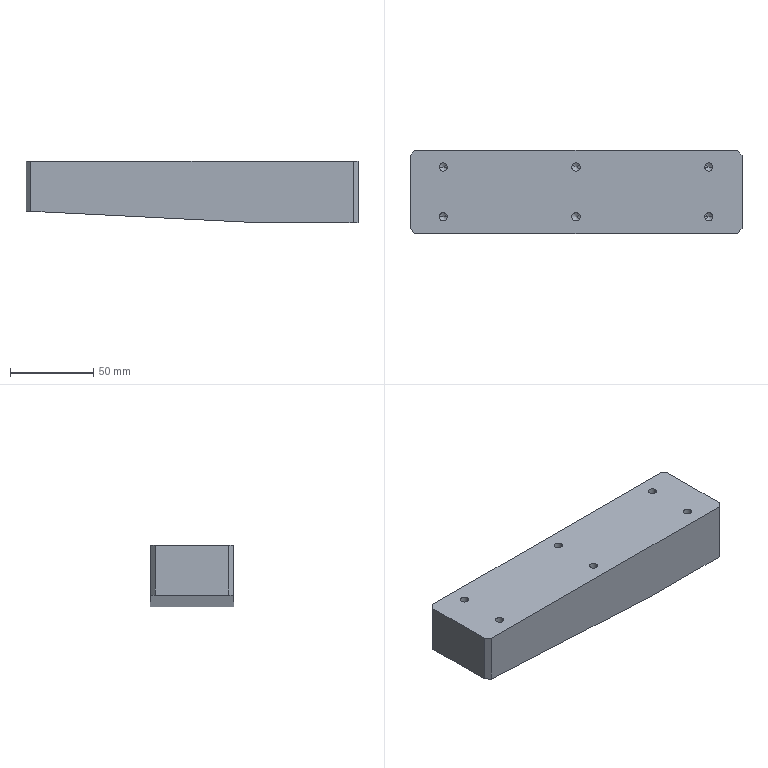Part | SolidWorks | features BaseBody 1 | 1 solid | 35 faces | box 200 x 50 x 37 mm | volume 343070 mm3 | cylinder 12 | cone 12 | plane 11 | commonest cylinder face diameters 5 x12
STEP:
#1=CARTESIAN_POINT('',(-82.5,15.,3.5));
#2=VERTEX_POINT('',#1);
#3=CARTESIAN_POINT('',(-77.5,15.,3.5));
#4=VERTEX_POINT('',#3);
#5=CARTESIAN_POINT('',(-80.,15.,3.5));
#6=DIRECTION('',(0.,0.,1.));
#7=DIRECTION('',(1.,0.,0.));
#8=AXIS2_PLACEMENT_3D('',#5,#6,#7);
#9=CIRCLE('',#8,2.5);
#10=EDGE_CURVE('',#2,#4,#9,.T.);
#11=ORIENTED_EDGE('',*,*,#10,.F.);
#12=CARTESIAN_POINT('',(-82.5,15.,18.5));
#13=VERTEX_POINT('',#12);
#14=CARTESIAN_POINT('',(-82.5,15.,18.5));
#15=DIRECTION('',(0.,0.,1.));
#16=VECTOR('',#15,1000.);
#17=LINE('',#14,#16);
#18=EDGE_CURVE('',#2,#13,#17,.T.);
#19=ORIENTED_EDGE('',*,*,#18,.T.);
#20=CARTESIAN_POINT('',(-77.5,15.,18.5));
#21=VERTEX_POINT('',#20);
#22=CARTESIAN_POINT('',(-80.,15.,18.5));
#23=DIRECTION('',(0.,0.,1.));
#24=DIRECTION('',(1.,0.,0.));
#25=AXIS2_PLACEMENT_3D('',#22,#23,#24);
#26=CIRCLE('',#25,2.5);
#27=EDGE_CURVE('',#13,#21,#26,.T.);
#28=ORIENTED_EDGE('',*,*,#27,.T.);
#29=CARTESIAN_POINT('',(-77.5,15.,18.5));
#30=DIRECTION('',(0.,0.,1.));
#31=VECTOR('',#30,1000.);
#32=LINE('',#29,#31);
#33=EDGE_CURVE('',#4,#21,#32,.T.);
#34=ORIENTED_EDGE('',*,*,#33,.F.);
#35=EDGE_LOOP('',(#11,#19,#28,#34));
#36=FACE_OUTER_BOUND('',#35,.T.);
#37=CARTESIAN_POINT('',(-80.,15.,18.5));
#38=DIRECTION('',(0.,0.,1.));
#39=DIRECTION('',(1.,0.,0.));
#40=AXIS2_PLACEMENT_3D('',#37,#38,#39);
#41=CYLINDRICAL_SURFACE('',#40,2.5);
#42=ADVANCED_FACE('',(#36),#41,.F.);
#43=CARTESIAN_POINT('',(-80.,15.,1.998));
#44=VERTEX_POINT('',#43);
#45=CARTESIAN_POINT('',(-77.5,15.,3.5));
#46=DIRECTION('',(0.8572,0.,0.515));
#47=VECTOR('',#46,1000.);
#48=LINE('',#45,#47);
#49=EDGE_CURVE('',#44,#4,#48,.T.);
#50=ORIENTED_EDGE('',*,*,#49,.F.);
#51=CARTESIAN_POINT('',(-82.5,15.,3.5));
#52=DIRECTION('',(-0.8572,0.,0.515));
#53=VECTOR('',#52,1000.);
#54=LINE('',#51,#53);
#55=EDGE_CURVE('',#44,#2,#54,.T.);
#56=ORIENTED_EDGE('',*,*,#55,.T.);
#57=ORIENTED_EDGE('',*,*,#10,.T.);
#58=EDGE_LOOP('',(#50,#56,#57));
#59=FACE_OUTER_BOUND('',#58,.T.);
#60=CARTESIAN_POINT('',(-80.,15.,3.5));
#61=DIRECTION('',(0.,0.,1.));
#62=DIRECTION('',(1.,0.,0.));
#63=AXIS2_PLACEMENT_3D('',#60,#61,#62);
#64=CONICAL_SURFACE('',#63,2.5,1.03);
#65=ADVANCED_FACE('',(#59),#64,.F.);
#66=CARTESIAN_POINT('',(-82.5,-15.,3.5));
#67=VERTEX_POINT('',#66);
#68=CARTESIAN_POINT('',(-77.5,-15.,3.5));
#69=VERTEX_POINT('',#68);
#70=CARTESIAN_POINT('',(-80.,-15.,3.5));
#71=DIRECTION('',(0.,0.,1.));
#72=DIRECTION('',(1.,0.,0.));
#73=AXIS2_PLACEMENT_3D('',#70,#71,#72);
#74=CIRCLE('',#73,2.5);
#75=EDGE_CURVE('',#67,#69,#74,.T.);
#76=ORIENTED_EDGE('',*,*,#75,.F.);
#77=CARTESIAN_POINT('',(-82.5,-15.,18.5));
#78=VERTEX_POINT('',#77);
#79=CARTESIAN_POINT('',(-82.5,-15.,18.5));
#80=DIRECTION('',(0.,0.,1.));
#81=VECTOR('',#80,1000.);
#82=LINE('',#79,#81);
#83=EDGE_CURVE('',#67,#78,#82,.T.);
#84=ORIENTED_EDGE('',*,*,#83,.T.);
#85=CARTESIAN_POINT('',(-77.5,-15.,18.5));
#86=VERTEX_POINT('',#85);
#87=CARTESIAN_POINT('',(-80.,-15.,18.5));
#88=DIRECTION('',(0.,0.,1.));
#89=DIRECTION('',(1.,0.,0.));
#90=AXIS2_PLACEMENT_3D('',#87,#88,#89);
#91=CIRCLE('',#90,2.5);
#92=EDGE_CURVE('',#78,#86,#91,.T.);
#93=ORIENTED_EDGE('',*,*,#92,.T.);
#94=CARTESIAN_POINT('',(-77.5,-15.,18.5));
#95=DIRECTION('',(0.,0.,1.));
#96=VECTOR('',#95,1000.);
#97=LINE('',#94,#96);
#98=EDGE_CURVE('',#69,#86,#97,.T.);
#99=ORIENTED_EDGE('',*,*,#98,.F.);
#100=EDGE_LOOP('',(#76,#84,#93,#99));
#101=FACE_OUTER_BOUND('',#100,.T.);
#102=CARTESIAN_POINT('',(-80.,-15.,18.5));
#103=DIRECTION('',(0.,0.,1.));
#104=DIRECTION('',(1.,0.,0.));
#105=AXIS2_PLACEMENT_3D('',#102,#103,#104);
#106=CYLINDRICAL_SURFACE('',#105,2.5);
#107=ADVANCED_FACE('',(#101),#106,.F.);
#108=CARTESIAN_POINT('',(-80.,-15.,1.998));
#109=VERTEX_POINT('',#108);
#110=CARTESIAN_POINT('',(-77.5,-15.,3.5));
#111=DIRECTION('',(0.8572,0.,0.515));
#112=VECTOR('',#111,1000.);
#113=LINE('',#110,#112);
#114=EDGE_CURVE('',#109,#69,#113,.T.);
#115=ORIENTED_EDGE('',*,*,#114,.F.);
#116=CARTESIAN_POINT('',(-82.5,-15.,3.5));
#117=DIRECTION('',(-0.8572,0.,0.515));
#118=VECTOR('',#117,1000.);
#119=LINE('',#116,#118);
#120=EDGE_CURVE('',#109,#67,#119,.T.);
#121=ORIENTED_EDGE('',*,*,#120,.T.);
#122=ORIENTED_EDGE('',*,*,#75,.T.);
#123=EDGE_LOOP('',(#115,#121,#122));
#124=FACE_OUTER_BOUND('',#123,.T.);
#125=CARTESIAN_POINT('',(-80.,-15.,3.5));
#126=DIRECTION('',(0.,0.,1.));
#127=DIRECTION('',(1.,0.,0.));
#128=AXIS2_PLACEMENT_3D('',#125,#126,#127);
#129=CONICAL_SURFACE('',#128,2.5,1.03);
#130=ADVANCED_FACE('',(#124),#129,.F.);
#131=CARTESIAN_POINT('',(-2.5,15.,3.5));
#132=VERTEX_POINT('',#131);
#133=CARTESIAN_POINT('',(2.5,15.,3.5));
#134=VERTEX_POINT('',#133);
#135=CARTESIAN_POINT('',(0.,15.,3.5));
#136=DIRECTION('',(0.,0.,1.));
#137=DIRECTION('',(1.,0.,0.));
#138=AXIS2_PLACEMENT_3D('',#135,#136,#137);
#139=CIRCLE('',#138,2.5);
#140=EDGE_CURVE('',#132,#134,#139,.T.);
#141=ORIENTED_EDGE('',*,*,#140,.F.);
#142=CARTESIAN_POINT('',(-2.5,15.,18.5));
#143=VERTEX_POINT('',#142);
#144=CARTESIAN_POINT('',(-2.5,15.,18.5));
#145=DIRECTION('',(0.,0.,1.));
#146=VECTOR('',#145,1000.);
#147=LINE('',#144,#146);
#148=EDGE_CURVE('',#132,#143,#147,.T.);
#149=ORIENTED_EDGE('',*,*,#148,.T.);
#150=CARTESIAN_POINT('',(2.5,15.,18.5));
#151=VERTEX_POINT('',#150);
#152=CARTESIAN_POINT('',(0.,15.,18.5));
#153=DIRECTION('',(0.,0.,1.));
#154=DIRECTION('',(1.,0.,0.));
#155=AXIS2_PLACEMENT_3D('',#152,#153,#154);
#156=CIRCLE('',#155,2.5);
#157=EDGE_CURVE('',#143,#151,#156,.T.);
#158=ORIENTED_EDGE('',*,*,#157,.T.);
#159=CARTESIAN_POINT('',(2.5,15.,18.5));
#160=DIRECTION('',(0.,0.,1.));
#161=VECTOR('',#160,1000.);
#162=LINE('',#159,#161);
#163=EDGE_CURVE('',#134,#151,#162,.T.);
#164=ORIENTED_EDGE('',*,*,#163,.F.);
#165=EDGE_LOOP('',(#141,#149,#158,#164));
#166=FACE_OUTER_BOUND('',#165,.T.);
#167=CARTESIAN_POINT('',(0.,15.,18.5));
#168=DIRECTION('',(0.,0.,1.));
#169=DIRECTION('',(1.,0.,0.));
#170=AXIS2_PLACEMENT_3D('',#167,#168,#169);
#171=CYLINDRICAL_SURFACE('',#170,2.5);
#172=ADVANCED_FACE('',(#166),#171,.F.);
#173=CARTESIAN_POINT('',(0.,15.,1.998));
#174=VERTEX_POINT('',#173);
#175=CARTESIAN_POINT('',(2.5,15.,3.5));
#176=DIRECTION('',(0.8572,0.,0.515));
#177=VECTOR('',#176,1000.);
#178=LINE('',#175,#177);
#179=EDGE_CURVE('',#174,#134,#178,.T.);
#180=ORIENTED_EDGE('',*,*,#179,.F.);
#181=CARTESIAN_POINT('',(-2.5,15.,3.5));
#182=DIRECTION('',(-0.8572,0.,0.515));
#183=VECTOR('',#182,1000.);
#184=LINE('',#181,#183);
#185=EDGE_CURVE('',#174,#132,#184,.T.);
#186=ORIENTED_EDGE('',*,*,#185,.T.);
#187=ORIENTED_EDGE('',*,*,#140,.T.);
#188=EDGE_LOOP('',(#180,#186,#187));
#189=FACE_OUTER_BOUND('',#188,.T.);
#190=CARTESIAN_POINT('',(0.,15.,3.5));
#191=DIRECTION('',(0.,0.,1.));
#192=DIRECTION('',(1.,0.,0.));
#193=AXIS2_PLACEMENT_3D('',#190,#191,#192);
#194=CONICAL_SURFACE('',#193,2.5,1.03);
#195=ADVANCED_FACE('',(#189),#194,.F.);
#196=CARTESIAN_POINT('',(-2.5,-15.,3.5));
#197=VERTEX_POINT('',#196);
#198=CARTESIAN_POINT('',(2.5,-15.,3.5));
#199=VERTEX_POINT('',#198);
#200=CARTESIAN_POINT('',(0.,-15.,3.5));
#201=DIRECTION('',(0.,0.,1.));
#202=DIRECTION('',(1.,0.,0.));
#203=AXIS2_PLACEMENT_3D('',#200,#201,#202);
#204=CIRCLE('',#203,2.5);
#205=EDGE_CURVE('',#197,#199,#204,.T.);
#206=ORIENTED_EDGE('',*,*,#205,.F.);
#207=CARTESIAN_POINT('',(-2.5,-15.,18.5));
#208=VERTEX_POINT('',#207);
#209=CARTESIAN_POINT('',(-2.5,-15.,18.5));
#210=DIRECTION('',(0.,0.,1.));
#211=VECTOR('',#210,1000.);
#212=LINE('',#209,#211);
#213=EDGE_CURVE('',#197,#208,#212,.T.);
#214=ORIENTED_EDGE('',*,*,#213,.T.);
#215=CARTESIAN_POINT('',(2.5,-15.,18.5));
#216=VERTEX_POINT('',#215);
#217=CARTESIAN_POINT('',(0.,-15.,18.5));
#218=DIRECTION('',(0.,0.,1.));
#219=DIRECTION('',(1.,0.,0.));
#220=AXIS2_PLACEMENT_3D('',#217,#218,#219);
#221=CIRCLE('',#220,2.5);
#222=EDGE_CURVE('',#208,#216,#221,.T.);
#223=ORIENTED_EDGE('',*,*,#222,.T.);
#224=CARTESIAN_POINT('',(2.5,-15.,18.5));
#225=DIRECTION('',(0.,0.,1.));
#226=VECTOR('',#225,1000.);
#227=LINE('',#224,#226);
#228=EDGE_CURVE('',#199,#216,#227,.T.);
#229=ORIENTED_EDGE('',*,*,#228,.F.);
#230=EDGE_LOOP('',(#206,#214,#223,#229));
#231=FACE_OUTER_BOUND('',#230,.T.);
#232=CARTESIAN_POINT('',(0.,-15.,18.5));
#233=DIRECTION('',(0.,0.,1.));
#234=DIRECTION('',(1.,0.,0.));
#235=AXIS2_PLACEMENT_3D('',#232,#233,#234);
#236=CYLINDRICAL_SURFACE('',#235,2.5);
#237=ADVANCED_FACE('',(#231),#236,.F.);
#238=CARTESIAN_POINT('',(0.,-15.,1.998));
#239=VERTEX_POINT('',#238);
#240=CARTESIAN_POINT('',(2.5,-15.,3.5));
#241=DIRECTION('',(0.8572,0.,0.515));
#242=VECTOR('',#241,1000.);
#243=LINE('',#240,#242);
#244=EDGE_CURVE('',#239,#199,#243,.T.);
#245=ORIENTED_EDGE('',*,*,#244,.F.);
#246=CARTESIAN_POINT('',(-2.5,-15.,3.5));
#247=DIRECTION('',(-0.8572,0.,0.515));
#248=VECTOR('',#247,1000.);
#249=LINE('',#246,#248);
#250=EDGE_CURVE('',#239,#197,#249,.T.);
#251=ORIENTED_EDGE('',*,*,#250,.T.);
#252=ORIENTED_EDGE('',*,*,#205,.T.);
#253=EDGE_LOOP('',(#245,#251,#252));
#254=FACE_OUTER_BOUND('',#253,.T.);
#255=CARTESIAN_POINT('',(0.,-15.,3.5));
#256=DIRECTION('',(0.,0.,1.));
#257=DIRECTION('',(1.,0.,0.));
#258=AXIS2_PLACEMENT_3D('',#255,#256,#257);
#259=CONICAL_SURFACE('',#258,2.5,1.03);
#260=ADVANCED_FACE('',(#254),#259,.F.);
#261=CARTESIAN_POINT('',(77.5,15.,3.5));
#262=VERTEX_POINT('',#261);
#263=CARTESIAN_POINT('',(82.5,15.,3.5));
#264=VERTEX_POINT('',#263);
#265=CARTESIAN_POINT('',(80.,15.,3.5));
#266=DIRECTION('',(0.,0.,1.));
#267=DIRECTION('',(1.,0.,0.));
#268=AXIS2_PLACEMENT_3D('',#265,#266,#267);
#269=CIRCLE('',#268,2.5);
#270=EDGE_CURVE('',#262,#264,#269,.T.);
#271=ORIENTED_EDGE('',*,*,#270,.F.);
#272=CARTESIAN_POINT('',(77.5,15.,18.5));
#273=VERTEX_POINT('',#272);
#274=CARTESIAN_POINT('',(77.5,15.,18.5));
#275=DIRECTION('',(0.,0.,1.));
#276=VECTOR('',#275,1000.);
#277=LINE('',#274,#276);
#278=EDGE_CURVE('',#262,#273,#277,.T.);
#279=ORIENTED_EDGE('',*,*,#278,.T.);
#280=CARTESIAN_POINT('',(82.5,15.,18.5));
#281=VERTEX_POINT('',#280);
#282=CARTESIAN_POINT('',(80.,15.,18.5));
#283=DIRECTION('',(0.,0.,1.));
#284=DIRECTION('',(1.,0.,0.));
#285=AXIS2_PLACEMENT_3D('',#282,#283,#284);
#286=CIRCLE('',#285,2.5);
#287=EDGE_CURVE('',#273,#281,#286,.T.);
#288=ORIENTED_EDGE('',*,*,#287,.T.);
#289=CARTESIAN_POINT('',(82.5,15.,18.5));
#290=DIRECTION('',(0.,0.,1.));
#291=VECTOR('',#290,1000.);
#292=LINE('',#289,#291);
#293=EDGE_CURVE('',#264,#281,#292,.T.);
#294=ORIENTED_EDGE('',*,*,#293,.F.);
#295=EDGE_LOOP('',(#271,#279,#288,#294));
#296=FACE_OUTER_BOUND('',#295,.T.);
#297=CARTESIAN_POINT('',(80.,15.,18.5));
#298=DIRECTION('',(0.,0.,1.));
#299=DIRECTION('',(1.,0.,0.));
#300=AXIS2_PLACEMENT_3D('',#297,#298,#299);
#301=CYLINDRICAL_SURFACE('',#300,2.5);
#302=ADVANCED_FACE('',(#296),#301,.F.);
#303=CARTESIAN_POINT('',(80.,15.,1.998));
#304=VERTEX_POINT('',#303);
#305=CARTESIAN_POINT('',(82.5,15.,3.5));
#306=DIRECTION('',(0.8572,0.,0.515));
#307=VECTOR('',#306,1000.);
#308=LINE('',#305,#307);
#309=EDGE_CURVE('',#304,#264,#308,.T.);
#310=ORIENTED_EDGE('',*,*,#309,.F.);
#311=CARTESIAN_POINT('',(77.5,15.,3.5));
#312=DIRECTION('',(-0.8572,0.,0.515));
#313=VECTOR('',#312,1000.);
#314=LINE('',#311,#313);
#315=EDGE_CURVE('',#304,#262,#314,.T.);
#316=ORIENTED_EDGE('',*,*,#315,.T.);
#317=ORIENTED_EDGE('',*,*,#270,.T.);
#318=EDGE_LOOP('',(#310,#316,#317));
#319=FACE_OUTER_BOUND('',#318,.T.);
#320=CARTESIAN_POINT('',(80.,15.,3.5));
#321=DIRECTION('',(0.,0.,1.));
#322=DIRECTION('',(1.,0.,0.));
#323=AXIS2_PLACEMENT_3D('',#320,#321,#322);
#324=CONICAL_SURFACE('',#323,2.5,1.03);
#325=ADVANCED_FACE('',(#319),#324,.F.);
#326=CARTESIAN_POINT('',(77.5,-15.,3.5));
#327=VERTEX_POINT('',#326);
#328=CARTESIAN_POINT('',(82.5,-15.,3.5));
#329=VERTEX_POINT('',#328);
#330=CARTESIAN_POINT('',(80.,-15.,3.5));
#331=DIRECTION('',(0.,0.,1.));
#332=DIRECTION('',(1.,0.,0.));
#333=AXIS2_PLACEMENT_3D('',#330,#331,#332);
#334=CIRCLE('',#333,2.5);
#335=EDGE_CURVE('',#327,#329,#334,.T.);
#336=ORIENTED_EDGE('',*,*,#335,.F.);
#337=CARTESIAN_POINT('',(77.5,-15.,18.5));
#338=VERTEX_POINT('',#337);
#339=CARTESIAN_POINT('',(77.5,-15.,18.5));
#340=DIRECTION('',(0.,0.,1.));
#341=VECTOR('',#340,1000.);
#342=LINE('',#339,#341);
#343=EDGE_CURVE('',#327,#338,#342,.T.);
#344=ORIENTED_EDGE('',*,*,#343,.T.);
#345=CARTESIAN_POINT('',(82.5,-15.,18.5));
#346=VERTEX_POINT('',#345);
#347=CARTESIAN_POINT('',(80.,-15.,18.5));
#348=DIRECTION('',(0.,0.,1.));
#349=DIRECTION('',(1.,0.,0.));
#350=AXIS2_PLACEMENT_3D('',#347,#348,#349);
#351=CIRCLE('',#350,2.5);
#352=EDGE_CURVE('',#338,#346,#351,.T.);
#353=ORIENTED_EDGE('',*,*,#352,.T.);
#354=CARTESIAN_POINT('',(82.5,-15.,18.5));
#355=DIRECTION('',(0.,0.,1.));
#356=VECTOR('',#355,1000.);
#357=LINE('',#354,#356);
#358=EDGE_CURVE('',#329,#346,#357,.T.);
#359=ORIENTED_EDGE('',*,*,#358,.F.);
#360=EDGE_LOOP('',(#336,#344,#353,#359));
#361=FACE_OUTER_BOUND('',#360,.T.);
#362=CARTESIAN_POINT('',(80.,-15.,18.5));
#363=DIRECTION('',(0.,0.,1.));
#364=DIRECTION('',(1.,0.,0.));
#365=AXIS2_PLACEMENT_3D('',#362,#363,#364);
#366=CYLINDRICAL_SURFACE('',#365,2.5);
#367=ADVANCED_FACE('',(#361),#366,.F.);
#368=CARTESIAN_POINT('',(80.,-15.,1.998));
#369=VERTEX_POINT('',#368);
#370=CARTESIAN_POINT('',(82.5,-15.,3.5));
#371=DIRECTION('',(0.8572,0.,0.515));
#372=VECTOR('',#371,1000.);
#373=LINE('',#370,#372);
#374=EDGE_CURVE('',#369,#329,#373,.T.);
#375=ORIENTED_EDGE('',*,*,#374,.F.);
#376=CARTESIAN_POINT('',(77.5,-15.,3.5));
#377=DIRECTION('',(-0.8572,0.,0.515));
#378=VECTOR('',#377,1000.);
#379=LINE('',#376,#378);
#380=EDGE_CURVE('',#369,#327,#379,.T.);
#381=ORIENTED_EDGE('',*,*,#380,.T.);
#382=ORIENTED_EDGE('',*,*,#335,.T.);
#383=EDGE_LOOP('',(#375,#381,#382));
#384=FACE_OUTER_BOUND('',#383,.T.);
#385=CARTESIAN_POINT('',(80.,-15.,3.5));
#386=DIRECTION('',(0.,0.,1.));
#387=DIRECTION('',(1.,0.,0.));
#388=AXIS2_PLACEMENT_3D('',#385,#386,#387);
#389=CONICAL_SURFACE('',#388,2.5,1.03);
#390=ADVANCED_FACE('',(#384),#389,.F.);
#391=CARTESIAN_POINT('',(-100.,-22.,-11.5));
#392=VERTEX_POINT('',#391);
#393=CARTESIAN_POINT('',(-100.,22.,-11.5));
#394=VERTEX_POINT('',#393);
#395=CARTESIAN_POINT('',(-100.,-25.,-11.5));
#396=DIRECTION('',(0.,1.,0.));
#397=VECTOR('',#396,1000.);
#398=LINE('',#395,#397);
#399=EDGE_CURVE('',#392,#394,#398,.T.);
#400=ORIENTED_EDGE('',*,*,#399,.F.);
#401=CARTESIAN_POINT('',(-100.,-22.,18.5));
#402=VERTEX_POINT('',#401);
#403=CARTESIAN_POINT('',(-100.,-22.,18.5));
#404=DIRECTION('',(0.,0.,1.));
#405=VECTOR('',#404,1000.);
#406=LINE('',#403,#405);
#407=EDGE_CURVE('',#392,#402,#406,.T.);
#408=ORIENTED_EDGE('',*,*,#407,.T.);
#409=CARTESIAN_POINT('',(-100.,22.,18.5));
#410=VERTEX_POINT('',#409);
#411=CARTESIAN_POINT('',(-100.,25.,18.5));
#412=DIRECTION('',(0.,-1.,0.));
#413=VECTOR('',#412,1000.);
#414=LINE('',#411,#413);
#415=EDGE_CURVE('',#410,#402,#414,.T.);
#416=ORIENTED_EDGE('',*,*,#415,.F.);
#417=CARTESIAN_POINT('',(-100.,22.,18.5));
#418=DIRECTION('',(0.,0.,-1.));
#419=VECTOR('',#418,1000.);
#420=LINE('',#417,#419);
#421=EDGE_CURVE('',#410,#394,#420,.T.);
#422=ORIENTED_EDGE('',*,*,#421,.T.);
#423=EDGE_LOOP('',(#400,#408,#416,#422));
#424=FACE_OUTER_BOUND('',#423,.T.);
#425=CARTESIAN_POINT('',(-100.,25.,18.5));
#426=DIRECTION('',(1.,0.,0.));
#427=DIRECTION('',(0.,0.,-1.));
#428=AXIS2_PLACEMENT_3D('',#425,#426,#427);
#429=PLANE('',#428);
#430=ADVANCED_FACE('',(#424),#429,.F.);
#431=CARTESIAN_POINT('',(40.,-25.,-18.5));
#432=VERTEX_POINT('',#431);
#433=CARTESIAN_POINT('',(97.,-25.,-18.5));
#434=VERTEX_POINT('',#433);
#435=CARTESIAN_POINT('',(100.,-25.,-18.5));
#436=DIRECTION('',(1.,0.,0.));
#437=VECTOR('',#436,1000.);
#438=LINE('',#435,#437);
#439=EDGE_CURVE('',#432,#434,#438,.T.);
#440=ORIENTED_EDGE('',*,*,#439,.T.);
#441=CARTESIAN_POINT('',(97.,-25.,18.5));
#442=VERTEX_POINT('',#441);
#443=CARTESIAN_POINT('',(97.,-25.,18.5));
#444=DIRECTION('',(0.,0.,1.));
#445=VECTOR('',#444,1000.);
#446=LINE('',#443,#445);
#447=EDGE_CURVE('',#434,#442,#446,.T.);
#448=ORIENTED_EDGE('',*,*,#447,.T.);
#449=CARTESIAN_POINT('',(-97.,-25.,18.5));
#450=VERTEX_POINT('',#449);
#451=CARTESIAN_POINT('',(100.,-25.,18.5));
#452=DIRECTION('',(1.,0.,0.));
#453=VECTOR('',#452,1000.);
#454=LINE('',#451,#453);
#455=EDGE_CURVE('',#450,#442,#454,.T.);
#456=ORIENTED_EDGE('',*,*,#455,.F.);
#457=CARTESIAN_POINT('',(-97.,-25.,-11.65));
#458=VERTEX_POINT('',#457);
#459=CARTESIAN_POINT('',(-97.,-25.,18.5));
#460=DIRECTION('',(0.,0.,-1.));
#461=VECTOR('',#460,1000.);
#462=LINE('',#459,#461);
#463=EDGE_CURVE('',#450,#458,#462,.T.);
#464=ORIENTED_EDGE('',*,*,#463,.T.);
#465=CARTESIAN_POINT('',(-100.,-25.,-11.5));
#466=DIRECTION('',(0.9988,0.,-0.04994));
#467=VECTOR('',#466,1000.);
#468=LINE('',#465,#467);
#469=EDGE_CURVE('',#458,#432,#468,.T.);
#470=ORIENTED_EDGE('',*,*,#469,.T.);
#471=EDGE_LOOP('',(#440,#448,#456,#464,#470));
#472=FACE_OUTER_BOUND('',#471,.T.);
#473=CARTESIAN_POINT('',(100.,-25.,18.5));
#474=DIRECTION('',(0.,1.,0.));
#475=DIRECTION('',(-1.,0.,0.));
#476=AXIS2_PLACEMENT_3D('',#473,#474,#475);
#477=PLANE('',#476);
#478=ADVANCED_FACE('',(#472),#477,.F.);
#479=CARTESIAN_POINT('',(100.,-22.,18.5));
#480=VERTEX_POINT('',#479);
#481=CARTESIAN_POINT('',(100.,22.,18.5));
#482=VERTEX_POINT('',#481);
#483=CARTESIAN_POINT('',(100.,25.,18.5));
#484=DIRECTION('',(0.,1.,0.));
#485=VECTOR('',#484,1000.);
#486=LINE('',#483,#485);
#487=EDGE_CURVE('',#480,#482,#486,.T.);
#488=ORIENTED_EDGE('',*,*,#487,.F.);
#489=CARTESIAN_POINT('',(100.,-22.,-18.5));
#490=VERTEX_POINT('',#489);
#491=CARTESIAN_POINT('',(100.,-22.,18.5));
#492=DIRECTION('',(0.,0.,-1.));
#493=VECTOR('',#492,1000.);
#494=LINE('',#491,#493);
#495=EDGE_CURVE('',#480,#490,#494,.T.);
#496=ORIENTED_EDGE('',*,*,#495,.T.);
#497=CARTESIAN_POINT('',(100.,22.,-18.5));
#498=VERTEX_POINT('',#497);
#499=CARTESIAN_POINT('',(100.,25.,-18.5));
#500=DIRECTION('',(0.,1.,0.));
#501=VECTOR('',#500,1000.);
#502=LINE('',#499,#501);
#503=EDGE_CURVE('',#490,#498,#502,.T.);
#504=ORIENTED_EDGE('',*,*,#503,.T.);
#505=CARTESIAN_POINT('',(100.,22.,18.5));
#506=DIRECTION('',(0.,0.,1.));
#507=VECTOR('',#506,1000.);
#508=LINE('',#505,#507);
#509=EDGE_CURVE('',#498,#482,#508,.T.);
#510=ORIENTED_EDGE('',*,*,#509,.T.);
#511=EDGE_LOOP('',(#488,#496,#504,#510));
#512=FACE_OUTER_BOUND('',#511,.T.);
#513=CARTESIAN_POINT('',(100.,25.,18.5));
#514=DIRECTION('',(-1.,0.,0.));
#515=DIRECTION('',(0.,0.,1.));
#516=AXIS2_PLACEMENT_3D('',#513,#514,#515);
#517=PLANE('',#516);
#518=ADVANCED_FACE('',(#512),#517,.F.);
#519=CARTESIAN_POINT('',(97.,25.,18.5));
#520=VERTEX_POINT('',#519);
#521=CARTESIAN_POINT('',(-97.,25.,18.5));
#522=VERTEX_POINT('',#521);
#523=CARTESIAN_POINT('',(100.,25.,18.5));
#524=DIRECTION('',(-1.,0.,0.));
#525=VECTOR('',#524,1000.);
#526=LINE('',#523,#525);
#527=EDGE_CURVE('',#520,#522,#526,.T.);
#528=ORIENTED_EDGE('',*,*,#527,.F.);
#529=CARTESIAN_POINT('',(97.,25.,-18.5));
#530=VERTEX_POINT('',#529);
#531=CARTESIAN_POINT('',(97.,25.,18.5));
#532=DIRECTION('',(0.,0.,-1.));
#533=VECTOR('',#532,1000.);
#534=LINE('',#531,#533);
#535=EDGE_CURVE('',#520,#530,#534,.T.);
#536=ORIENTED_EDGE('',*,*,#535,.T.);
#537=CARTESIAN_POINT('',(40.,25.,-18.5));
#538=VERTEX_POINT('',#537);
#539=CARTESIAN_POINT('',(100.,25.,-18.5));
#540=DIRECTION('',(-1.,0.,0.));
#541=VECTOR('',#540,1000.);
#542=LINE('',#539,#541);
#543=EDGE_CURVE('',#530,#538,#542,.T.);
#544=ORIENTED_EDGE('',*,*,#543,.T.);
#545=CARTESIAN_POINT('',(-97.,25.,-11.65));
#546=VERTEX_POINT('',#545);
#547=CARTESIAN_POINT('',(-100.,25.,-11.5));
#548=DIRECTION('',(0.9988,0.,-0.04994));
#549=VECTOR('',#548,1000.);
#550=LINE('',#547,#549);
#551=EDGE_CURVE('',#546,#538,#550,.T.);
#552=ORIENTED_EDGE('',*,*,#551,.F.);
#553=CARTESIAN_POINT('',(-97.,25.,18.5));
#554=DIRECTION('',(0.,0.,1.));
#555=VECTOR('',#554,1000.);
#556=LINE('',#553,#555);
#557=EDGE_CURVE('',#546,#522,#556,.T.);
#558=ORIENTED_EDGE('',*,*,#557,.T.);
#559=EDGE_LOOP('',(#528,#536,#544,#552,#558));
#560=FACE_OUTER_BOUND('',#559,.T.);
#561=CARTESIAN_POINT('',(100.,25.,18.5));
#562=DIRECTION('',(0.,-1.,0.));
#563=DIRECTION('',(1.,0.,0.));
#564=AXIS2_PLACEMENT_3D('',#561,#562,#563);
#565=PLANE('',#564);
#566=ADVANCED_FACE('',(#560),#565,.F.);
#567=CARTESIAN_POINT('',(-80.,15.,18.5));
#568=DIRECTION('',(0.,0.,1.));
#569=DIRECTION('',(1.,0.,0.));
#570=AXIS2_PLACEMENT_3D('',#567,#568,#569);
#571=CIRCLE('',#570,2.5);
#572=EDGE_CURVE('',#21,#13,#571,.T.);
#573=ORIENTED_EDGE('',*,*,#572,.F.);
#574=ORIENTED_EDGE('',*,*,#27,.F.);
#575=EDGE_LOOP('',(#573,#574));
#576=FACE_BOUND('',#575,.T.);
#577=CARTESIAN_POINT('',(-80.,-15.,18.5));
#578=DIRECTION('',(0.,0.,1.));
#579=DIRECTION('',(1.,0.,0.));
#580=AXIS2_PLACEMENT_3D('',#577,#578,#579);
#581=CIRCLE('',#580,2.5);
#582=EDGE_CURVE('',#86,#78,#581,.T.);
#583=ORIENTED_EDGE('',*,*,#582,.F.);
#584=ORIENTED_EDGE('',*,*,#92,.F.);
#585=EDGE_LOOP('',(#583,#584));
#586=FACE_BOUND('',#585,.T.);
#587=CARTESIAN_POINT('',(0.,15.,18.5));
#588=DIRECTION('',(0.,0.,1.));
#589=DIRECTION('',(1.,0.,0.));
#590=AXIS2_PLACEMENT_3D('',#587,#588,#589);
#591=CIRCLE('',#590,2.5);
#592=EDGE_CURVE('',#151,#143,#591,.T.);
#593=ORIENTED_EDGE('',*,*,#592,.F.);
#594=ORIENTED_EDGE('',*,*,#157,.F.);
#595=EDGE_LOOP('',(#593,#594));
#596=FACE_BOUND('',#595,.T.);
#597=CARTESIAN_POINT('',(0.,-15.,18.5));
#598=DIRECTION('',(0.,0.,1.));
#599=DIRECTION('',(1.,0.,0.));
#600=AXIS2_PLACEMENT_3D('',#597,#598,#599);
#601=CIRCLE('',#600,2.5);
#602=EDGE_CURVE('',#216,#208,#601,.T.);
#603=ORIENTED_EDGE('',*,*,#602,.F.);
#604=ORIENTED_EDGE('',*,*,#222,.F.);
#605=EDGE_LOOP('',(#603,#604));
#606=FACE_BOUND('',#605,.T.);
#607=CARTESIAN_POINT('',(80.,15.,18.5));
#608=DIRECTION('',(0.,0.,1.));
#609=DIRECTION('',(1.,0.,0.));
#610=AXIS2_PLACEMENT_3D('',#607,#608,#609);
#611=CIRCLE('',#610,2.5);
#612=EDGE_CURVE('',#281,#273,#611,.T.);
#613=ORIENTED_EDGE('',*,*,#612,.F.);
#614=ORIENTED_EDGE('',*,*,#287,.F.);
#615=EDGE_LOOP('',(#613,#614));
#616=FACE_BOUND('',#615,.T.);
#617=CARTESIAN_POINT('',(80.,-15.,18.5));
#618=DIRECTION('',(0.,0.,1.));
#619=DIRECTION('',(1.,0.,0.));
#620=AXIS2_PLACEMENT_3D('',#617,#618,#619);
#621=CIRCLE('',#620,2.5);
#622=EDGE_CURVE('',#346,#338,#621,.T.);
#623=ORIENTED_EDGE('',*,*,#622,.F.);
#624=ORIENTED_EDGE('',*,*,#352,.F.);
#625=EDGE_LOOP('',(#623,#624));
#626=FACE_BOUND('',#625,.T.);
#627=ORIENTED_EDGE('',*,*,#455,.T.);
#628=CARTESIAN_POINT('',(100.,-22.,18.5));
#629=DIRECTION('',(0.7071,0.7071,0.));
#630=VECTOR('',#629,1000.);
#631=LINE('',#628,#630);
#632=EDGE_CURVE('',#442,#480,#631,.T.);
#633=ORIENTED_EDGE('',*,*,#632,.T.);
#634=ORIENTED_EDGE('',*,*,#487,.T.);
#635=CARTESIAN_POINT('',(97.,25.,18.5));
#636=DIRECTION('',(-0.7071,0.7071,0.));
#637=VECTOR('',#636,1000.);
#638=LINE('',#635,#637);
#639=EDGE_CURVE('',#482,#520,#638,.T.);
#640=ORIENTED_EDGE('',*,*,#639,.T.);
#641=ORIENTED_EDGE('',*,*,#527,.T.);
#642=CARTESIAN_POINT('',(-100.,22.,18.5));
#643=DIRECTION('',(-0.7071,-0.7071,0.));
#644=VECTOR('',#643,1000.);
#645=LINE('',#642,#644);
#646=EDGE_CURVE('',#522,#410,#645,.T.);
#647=ORIENTED_EDGE('',*,*,#646,.T.);
#648=ORIENTED_EDGE('',*,*,#415,.T.);
#649=CARTESIAN_POINT('',(-97.,-25.,18.5));
#650=DIRECTION('',(0.7071,-0.7071,0.));
#651=VECTOR('',#650,1000.);
#652=LINE('',#649,#651);
#653=EDGE_CURVE('',#402,#450,#652,.T.);
#654=ORIENTED_EDGE('',*,*,#653,.T.);
#655=EDGE_LOOP('',(#627,#633,#634,#640,#641,#647,#648,#654));
#656=FACE_OUTER_BOUND('',#655,.T.);
#657=CARTESIAN_POINT('',(-100.,-25.,18.5));
#658=DIRECTION('',(0.,0.,-1.));
#659=DIRECTION('',(-1.,0.,0.));
#660=AXIS2_PLACEMENT_3D('',#657,#658,#659);
#661=PLANE('',#660);
#662=ADVANCED_FACE('',(#576,#586,#596,#606,#616,#626,#656),#661,.F.);
#663=ORIENTED_EDGE('',*,*,#503,.F.);
#664=CARTESIAN_POINT('',(-1.5,-123.5,-18.5));
#665=DIRECTION('',(-0.7071,-0.7071,0.));
#666=VECTOR('',#665,1000.);
#667=LINE('',#664,#666);
#668=EDGE_CURVE('',#490,#434,#667,.T.);
#669=ORIENTED_EDGE('',*,*,#668,.T.);
#670=ORIENTED_EDGE('',*,*,#439,.F.);
#671=CARTESIAN_POINT('',(40.,-25.,-18.5));
#672=DIRECTION('',(0.,1.,0.));
#673=VECTOR('',#672,1000.);
#674=LINE('',#671,#673);
#675=EDGE_CURVE('',#432,#538,#674,.T.);
#676=ORIENTED_EDGE('',*,*,#675,.T.);
#677=ORIENTED_EDGE('',*,*,#543,.F.);
#678=CARTESIAN_POINT('',(23.5,98.5,-18.5));
#679=DIRECTION('',(0.7071,-0.7071,0.));
#680=VECTOR('',#679,1000.);
#681=LINE('',#678,#680);
#682=EDGE_CURVE('',#530,#498,#681,.T.);
#683=ORIENTED_EDGE('',*,*,#682,.T.);
#684=EDGE_LOOP('',(#663,#669,#670,#676,#677,#683));
#685=FACE_OUTER_BOUND('',#684,.T.);
#686=CARTESIAN_POINT('',(-100.,-25.,-18.5));
#687=DIRECTION('',(0.,0.,-1.));
#688=DIRECTION('',(-1.,0.,0.));
#689=AXIS2_PLACEMENT_3D('',#686,#687,#688);
#690=PLANE('',#689);
#691=ADVANCED_FACE('',(#685),#690,.T.);
#692=ORIENTED_EDGE('',*,*,#469,.F.);
#693=CARTESIAN_POINT('',(-97.753,-24.247,-11.612));
#694=DIRECTION('',(-0.7067,0.7067,0.03533));
#695=VECTOR('',#694,1000.);
#696=LINE('',#693,#695);
#697=EDGE_CURVE('',#458,#392,#696,.T.);
#698=ORIENTED_EDGE('',*,*,#697,.T.);
#699=ORIENTED_EDGE('',*,*,#399,.T.);
#700=CARTESIAN_POINT('',(-100.749,21.251,-11.463));
#701=DIRECTION('',(0.7067,0.7067,-0.03533));
#702=VECTOR('',#701,1000.);
#703=LINE('',#700,#702);
#704=EDGE_CURVE('',#394,#546,#703,.T.);
#705=ORIENTED_EDGE('',*,*,#704,.T.);
#706=ORIENTED_EDGE('',*,*,#551,.T.);
#707=ORIENTED_EDGE('',*,*,#675,.F.);
#708=EDGE_LOOP('',(#692,#698,#699,#705,#706,#707));
#709=FACE_OUTER_BOUND('',#708,.T.);
#710=CARTESIAN_POINT('',(-100.,-25.,-11.5));
#711=DIRECTION('',(0.04994,0.,0.9988));
#712=DIRECTION('',(0.9988,0.,-0.04994));
#713=AXIS2_PLACEMENT_3D('',#710,#711,#712);
#714=PLANE('',#713);
#715=ADVANCED_FACE('',(#709),#714,.F.);
#716=ORIENTED_EDGE('',*,*,#632,.F.);
#717=ORIENTED_EDGE('',*,*,#447,.F.);
#718=ORIENTED_EDGE('',*,*,#668,.F.);
#719=ORIENTED_EDGE('',*,*,#495,.F.);
#720=EDGE_LOOP('',(#716,#717,#718,#719));
#721=FACE_OUTER_BOUND('',#720,.T.);
#722=CARTESIAN_POINT('',(100.,-22.,18.5));
#723=DIRECTION('',(-0.7071,0.7071,0.));
#724=DIRECTION('',(-0.7071,-0.7071,0.));
#725=AXIS2_PLACEMENT_3D('',#722,#723,#724);
#726=PLANE('',#725);
#727=ADVANCED_FACE('',(#721),#726,.F.);
#728=ORIENTED_EDGE('',*,*,#639,.F.);
#729=ORIENTED_EDGE('',*,*,#509,.F.);
#730=ORIENTED_EDGE('',*,*,#682,.F.);
#731=ORIENTED_EDGE('',*,*,#535,.F.);
#732=EDGE_LOOP('',(#728,#729,#730,#731));
#733=FACE_OUTER_BOUND('',#732,.T.);
#734=CARTESIAN_POINT('',(97.,25.,18.5));
#735=DIRECTION('',(-0.7071,-0.7071,0.));
#736=DIRECTION('',(0.7071,-0.7071,0.));
#737=AXIS2_PLACEMENT_3D('',#734,#735,#736);
#738=PLANE('',#737);
#739=ADVANCED_FACE('',(#733),#738,.F.);
#740=ORIENTED_EDGE('',*,*,#653,.F.);
#741=ORIENTED_EDGE('',*,*,#407,.F.);
#742=ORIENTED_EDGE('',*,*,#697,.F.);
#743=ORIENTED_EDGE('',*,*,#463,.F.);
#744=EDGE_LOOP('',(#740,#741,#742,#743));
#745=FACE_OUTER_BOUND('',#744,.T.);
#746=CARTESIAN_POINT('',(-97.,-25.,18.5));
#747=DIRECTION('',(0.7071,0.7071,0.));
#748=DIRECTION('',(-0.7071,0.7071,0.));
#749=AXIS2_PLACEMENT_3D('',#746,#747,#748);
#750=PLANE('',#749);
#751=ADVANCED_FACE('',(#745),#750,.F.);
#752=ORIENTED_EDGE('',*,*,#646,.F.);
#753=ORIENTED_EDGE('',*,*,#557,.F.);
#754=ORIENTED_EDGE('',*,*,#704,.F.);
#755=ORIENTED_EDGE('',*,*,#421,.F.);
#756=EDGE_LOOP('',(#752,#753,#754,#755));
#757=FACE_OUTER_BOUND('',#756,.T.);
#758=CARTESIAN_POINT('',(-100.,22.,18.5));
#759=DIRECTION('',(0.7071,-0.7071,0.));
#760=DIRECTION('',(0.7071,0.7071,0.));
#761=AXIS2_PLACEMENT_3D('',#758,#759,#760);
#762=PLANE('',#761);
#763=ADVANCED_FACE('',(#757),#762,.F.);
#764=ORIENTED_EDGE('',*,*,#380,.F.);
#765=ORIENTED_EDGE('',*,*,#374,.T.);
#766=CARTESIAN_POINT('',(80.,-15.,3.5));
#767=DIRECTION('',(0.,0.,1.));
#768=DIRECTION('',(1.,0.,0.));
#769=AXIS2_PLACEMENT_3D('',#766,#767,#768);
#770=CIRCLE('',#769,2.5);
#771=EDGE_CURVE('',#329,#327,#770,.T.);
#772=ORIENTED_EDGE('',*,*,#771,.T.);
#773=EDGE_LOOP('',(#764,#765,#772));
#774=FACE_OUTER_BOUND('',#773,.T.);
#775=CARTESIAN_POINT('',(80.,-15.,3.5));
#776=DIRECTION('',(0.,0.,1.));
#777=DIRECTION('',(1.,0.,0.));
#778=AXIS2_PLACEMENT_3D('',#775,#776,#777);
#779=CONICAL_SURFACE('',#778,2.5,1.03);
#780=ADVANCED_FACE('',(#774),#779,.F.);
#781=ORIENTED_EDGE('',*,*,#343,.F.);
#782=ORIENTED_EDGE('',*,*,#771,.F.);
#783=ORIENTED_EDGE('',*,*,#358,.T.);
#784=ORIENTED_EDGE('',*,*,#622,.T.);
#785=EDGE_LOOP('',(#781,#782,#783,#784));
#786=FACE_OUTER_BOUND('',#785,.T.);
#787=CARTESIAN_POINT('',(80.,-15.,18.5));
#788=DIRECTION('',(0.,0.,1.));
#789=DIRECTION('',(1.,0.,0.));
#790=AXIS2_PLACEMENT_3D('',#787,#788,#789);
#791=CYLINDRICAL_SURFACE('',#790,2.5);
#792=ADVANCED_FACE('',(#786),#791,.F.);
#793=ORIENTED_EDGE('',*,*,#315,.F.);
#794=ORIENTED_EDGE('',*,*,#309,.T.);
#795=CARTESIAN_POINT('',(80.,15.,3.5));
#796=DIRECTION('',(0.,0.,1.));
#797=DIRECTION('',(1.,0.,0.));
#798=AXIS2_PLACEMENT_3D('',#795,#796,#797);
#799=CIRCLE('',#798,2.5);
#800=EDGE_CURVE('',#264,#262,#799,.T.);
#801=ORIENTED_EDGE('',*,*,#800,.T.);
#802=EDGE_LOOP('',(#793,#794,#801));
#803=FACE_OUTER_BOUND('',#802,.T.);
#804=CARTESIAN_POINT('',(80.,15.,3.5));
#805=DIRECTION('',(0.,0.,1.));
#806=DIRECTION('',(1.,0.,0.));
#807=AXIS2_PLACEMENT_3D('',#804,#805,#806);
#808=CONICAL_SURFACE('',#807,2.5,1.03);
#809=ADVANCED_FACE('',(#803),#808,.F.);
#810=ORIENTED_EDGE('',*,*,#278,.F.);
#811=ORIENTED_EDGE('',*,*,#800,.F.);
#812=ORIENTED_EDGE('',*,*,#293,.T.);
#813=ORIENTED_EDGE('',*,*,#612,.T.);
#814=EDGE_LOOP('',(#810,#811,#812,#813));
#815=FACE_OUTER_BOUND('',#814,.T.);
#816=CARTESIAN_POINT('',(80.,15.,18.5));
#817=DIRECTION('',(0.,0.,1.));
#818=DIRECTION('',(1.,0.,0.));
#819=AXIS2_PLACEMENT_3D('',#816,#817,#818);
#820=CYLINDRICAL_SURFACE('',#819,2.5);
#821=ADVANCED_FACE('',(#815),#820,.F.);
#822=ORIENTED_EDGE('',*,*,#250,.F.);
#823=ORIENTED_EDGE('',*,*,#244,.T.);
#824=CARTESIAN_POINT('',(0.,-15.,3.5));
#825=DIRECTION('',(0.,0.,1.));
#826=DIRECTION('',(1.,0.,0.));
#827=AXIS2_PLACEMENT_3D('',#824,#825,#826);
#828=CIRCLE('',#827,2.5);
#829=EDGE_CURVE('',#199,#197,#828,.T.);
#830=ORIENTED_EDGE('',*,*,#829,.T.);
#831=EDGE_LOOP('',(#822,#823,#830));
#832=FACE_OUTER_BOUND('',#831,.T.);
#833=CARTESIAN_POINT('',(0.,-15.,3.5));
#834=DIRECTION('',(0.,0.,1.));
#835=DIRECTION('',(1.,0.,0.));
#836=AXIS2_PLACEMENT_3D('',#833,#834,#835);
#837=CONICAL_SURFACE('',#836,2.5,1.03);
#838=ADVANCED_FACE('',(#832),#837,.F.);
#839=ORIENTED_EDGE('',*,*,#213,.F.);
#840=ORIENTED_EDGE('',*,*,#829,.F.);
#841=ORIENTED_EDGE('',*,*,#228,.T.);
#842=ORIENTED_EDGE('',*,*,#602,.T.);
#843=EDGE_LOOP('',(#839,#840,#841,#842));
#844=FACE_OUTER_BOUND('',#843,.T.);
#845=CARTESIAN_POINT('',(0.,-15.,18.5));
#846=DIRECTION('',(0.,0.,1.));
#847=DIRECTION('',(1.,0.,0.));
#848=AXIS2_PLACEMENT_3D('',#845,#846,#847);
#849=CYLINDRICAL_SURFACE('',#848,2.5);
#850=ADVANCED_FACE('',(#844),#849,.F.);
#851=ORIENTED_EDGE('',*,*,#185,.F.);
#852=ORIENTED_EDGE('',*,*,#179,.T.);
#853=CARTESIAN_POINT('',(0.,15.,3.5));
#854=DIRECTION('',(0.,0.,1.));
#855=DIRECTION('',(1.,0.,0.));
#856=AXIS2_PLACEMENT_3D('',#853,#854,#855);
#857=CIRCLE('',#856,2.5);
#858=EDGE_CURVE('',#134,#132,#857,.T.);
#859=ORIENTED_EDGE('',*,*,#858,.T.);
#860=EDGE_LOOP('',(#851,#852,#859));
#861=FACE_OUTER_BOUND('',#860,.T.);
#862=CARTESIAN_POINT('',(0.,15.,3.5));
#863=DIRECTION('',(0.,0.,1.));
#864=DIRECTION('',(1.,0.,0.));
#865=AXIS2_PLACEMENT_3D('',#862,#863,#864);
#866=CONICAL_SURFACE('',#865,2.5,1.03);
#867=ADVANCED_FACE('',(#861),#866,.F.);
#868=ORIENTED_EDGE('',*,*,#148,.F.);
#869=ORIENTED_EDGE('',*,*,#858,.F.);
#870=ORIENTED_EDGE('',*,*,#163,.T.);
#871=ORIENTED_EDGE('',*,*,#592,.T.);
#872=EDGE_LOOP('',(#868,#869,#870,#871));
#873=FACE_OUTER_BOUND('',#872,.T.);
#874=CARTESIAN_POINT('',(0.,15.,18.5));
#875=DIRECTION('',(0.,0.,1.));
#876=DIRECTION('',(1.,0.,0.));
#877=AXIS2_PLACEMENT_3D('',#874,#875,#876);
#878=CYLINDRICAL_SURFACE('',#877,2.5);
#879=ADVANCED_FACE('',(#873),#878,.F.);
#880=ORIENTED_EDGE('',*,*,#120,.F.);
#881=ORIENTED_EDGE('',*,*,#114,.T.);
#882=CARTESIAN_POINT('',(-80.,-15.,3.5));
#883=DIRECTION('',(0.,0.,1.));
#884=DIRECTION('',(1.,0.,0.));
#885=AXIS2_PLACEMENT_3D('',#882,#883,#884);
#886=CIRCLE('',#885,2.5);
#887=EDGE_CURVE('',#69,#67,#886,.T.);
#888=ORIENTED_EDGE('',*,*,#887,.T.);
#889=EDGE_LOOP('',(#880,#881,#888));
#890=FACE_OUTER_BOUND('',#889,.T.);
#891=CARTESIAN_POINT('',(-80.,-15.,3.5));
#892=DIRECTION('',(0.,0.,1.));
#893=DIRECTION('',(1.,0.,0.));
#894=AXIS2_PLACEMENT_3D('',#891,#892,#893);
#895=CONICAL_SURFACE('',#894,2.5,1.03);
#896=ADVANCED_FACE('',(#890),#895,.F.);
#897=ORIENTED_EDGE('',*,*,#83,.F.);
#898=ORIENTED_EDGE('',*,*,#887,.F.);
#899=ORIENTED_EDGE('',*,*,#98,.T.);
#900=ORIENTED_EDGE('',*,*,#582,.T.);
#901=EDGE_LOOP('',(#897,#898,#899,#900));
#902=FACE_OUTER_BOUND('',#901,.T.);
#903=CARTESIAN_POINT('',(-80.,-15.,18.5));
#904=DIRECTION('',(0.,0.,1.));
#905=DIRECTION('',(1.,0.,0.));
#906=AXIS2_PLACEMENT_3D('',#903,#904,#905);
#907=CYLINDRICAL_SURFACE('',#906,2.5);
#908=ADVANCED_FACE('',(#902),#907,.F.);
#909=ORIENTED_EDGE('',*,*,#55,.F.);
#910=ORIENTED_EDGE('',*,*,#49,.T.);
#911=CARTESIAN_POINT('',(-80.,15.,3.5));
#912=DIRECTION('',(0.,0.,1.));
#913=DIRECTION('',(1.,0.,0.));
#914=AXIS2_PLACEMENT_3D('',#911,#912,#913);
#915=CIRCLE('',#914,2.5);
#916=EDGE_CURVE('',#4,#2,#915,.T.);
#917=ORIENTED_EDGE('',*,*,#916,.T.);
#918=EDGE_LOOP('',(#909,#910,#917));
#919=FACE_OUTER_BOUND('',#918,.T.);
#920=CARTESIAN_POINT('',(-80.,15.,3.5));
#921=DIRECTION('',(0.,0.,1.));
#922=DIRECTION('',(1.,0.,0.));
#923=AXIS2_PLACEMENT_3D('',#920,#921,#922);
#924=CONICAL_SURFACE('',#923,2.5,1.03);
#925=ADVANCED_FACE('',(#919),#924,.F.);
#926=ORIENTED_EDGE('',*,*,#18,.F.);
#927=ORIENTED_EDGE('',*,*,#916,.F.);
#928=ORIENTED_EDGE('',*,*,#33,.T.);
#929=ORIENTED_EDGE('',*,*,#572,.T.);
#930=EDGE_LOOP('',(#926,#927,#928,#929));
#931=FACE_OUTER_BOUND('',#930,.T.);
#932=CARTESIAN_POINT('',(-80.,15.,18.5));
#933=DIRECTION('',(0.,0.,1.));
#934=DIRECTION('',(1.,0.,0.));
#935=AXIS2_PLACEMENT_3D('',#932,#933,#934);
#936=CYLINDRICAL_SURFACE('',#935,2.5);
#937=ADVANCED_FACE('',(#931),#936,.F.);
#938=CLOSED_SHELL('',(#42,#65,#107,#130,#172,#195,#237,#260,#302,#325,#367,#390,#430,#478,#518,#566,#662,#691,#715,#727,#739,#751,#763,#780,#792,#809,#821,#838,#850,#867,#879,#896,#908,#925,#937));
#939=MANIFOLD_SOLID_BREP('',#938);
#940=CARTESIAN_POINT('',(0.,0.,0.));
#941=DIRECTION('',(0.,0.,1.));
#942=DIRECTION('',(1.,0.,0.));
#943=AXIS2_PLACEMENT_3D('',#940,#941,#942);
#944=(LENGTH_UNIT()NAMED_UNIT(*)SI_UNIT(.MILLI.,.METRE.));
#945=UNCERTAINTY_MEASURE_WITH_UNIT(LENGTH_MEASURE(0.00001),#944,'','');
#946=(NAMED_UNIT(*)PLANE_ANGLE_UNIT()SI_UNIT($,.RADIAN.));
#947=(NAMED_UNIT(*)SI_UNIT($,.STERADIAN.)SOLID_ANGLE_UNIT());
#948=(GEOMETRIC_REPRESENTATION_CONTEXT(3)GLOBAL_UNCERTAINTY_ASSIGNED_CONTEXT((#945))GLOBAL_UNIT_ASSIGNED_CONTEXT((#944,#946,#947))REPRESENTATION_CONTEXT('',''));
#949=ADVANCED_BREP_SHAPE_REPRESENTATION('',(#939,#943),#948);